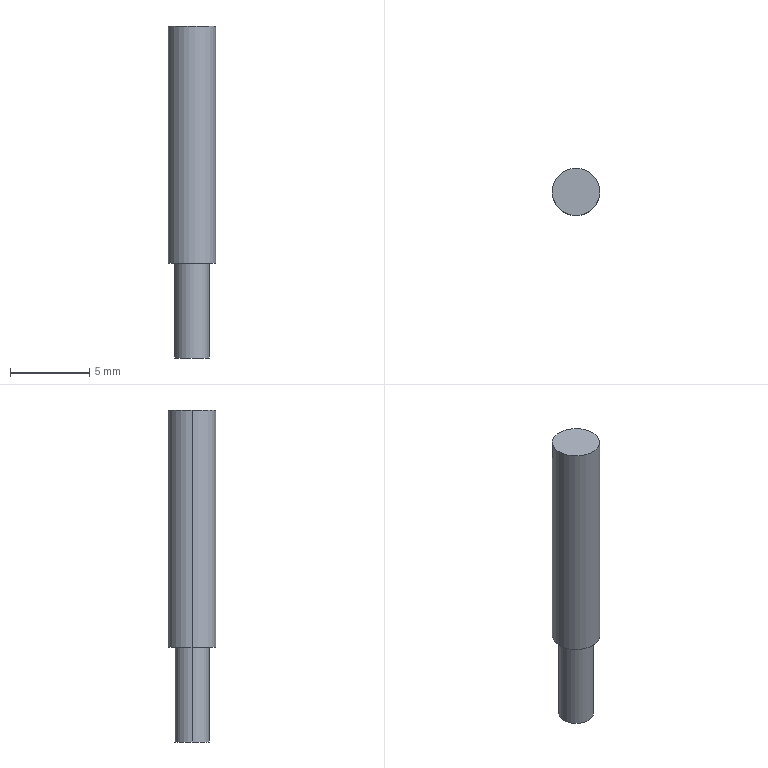Part | STEP file | through-beam fiber sensor FT-D321Q-M | 1 solid | 7 faces | box 3 x 3 x 21 mm | volume 128.837 mm3 | cylinder 4 | plane 3 | commonest cylinder face diameters 2.2 x2 3 x2
STEP:
#1=CARTESIAN_POINT('',(0.,0.,0.));
#2=DIRECTION('',(0.,0.,1.));
#3=DIRECTION('',(1.,0.,0.));
#4=AXIS2_PLACEMENT_3D('',#1,#2,#3);
#5=CARTESIAN_POINT('',(-1.1,0.,-6.));
#6=VERTEX_POINT('',#5);
#7=CARTESIAN_POINT('',(1.1,0.,-6.));
#8=VERTEX_POINT('',#7);
#9=CARTESIAN_POINT('',(0.,0.,-6.));
#10=DIRECTION('',(0.,0.,-1.));
#11=DIRECTION('',(-1.,0.,0.));
#12=AXIS2_PLACEMENT_3D('',#9,#10,#11);
#13=CIRCLE('',#12,1.1);
#14=CARTESIAN_POINT('',(0.,0.,-6.));
#15=DIRECTION('',(0.,0.,1.));
#16=DIRECTION('',(1.,0.,0.));
#17=AXIS2_PLACEMENT_3D('',#14,#15,#16);
#18=CYLINDRICAL_SURFACE('',#17,1.1);
#19=CARTESIAN_POINT('',(3.142,0.));
#20=DIRECTION('',(-1.,0.));
#21=VECTOR('',#20,1.);
#22=LINE('',#19,#21);
#23=(GEOMETRIC_REPRESENTATION_CONTEXT(2)PARAMETRIC_REPRESENTATION_CONTEXT()REPRESENTATION_CONTEXT('',''));
#24=DEFINITIONAL_REPRESENTATION('',(#22),#23);
#25=PCURVE('',#18,#24);
#26=CARTESIAN_POINT('',(0.,0.,-6.));
#27=DIRECTION('',(0.,0.,-1.));
#28=DIRECTION('',(-1.,0.,0.));
#29=AXIS2_PLACEMENT_3D('',#26,#27,#28);
#30=PLANE('',#29);
#31=CARTESIAN_POINT('',(0.,0.));
#32=DIRECTION('',(1.,0.));
#33=AXIS2_PLACEMENT_2D('',#31,#32);
#34=CIRCLE('',#33,1.1);
#35=(GEOMETRIC_REPRESENTATION_CONTEXT(2)PARAMETRIC_REPRESENTATION_CONTEXT()REPRESENTATION_CONTEXT('',''));
#36=DEFINITIONAL_REPRESENTATION('',(#34),#35);
#37=PCURVE('',#30,#36);
#38=SURFACE_CURVE('',#13,(#25,#37),.PCURVE_S1.);
#39=EDGE_CURVE('',#6,#8,#38,.T.);
#40=ORIENTED_EDGE('',*,*,#39,.F.);
#41=CARTESIAN_POINT('',(-1.1,0.,0.));
#42=VERTEX_POINT('',#41);
#43=CARTESIAN_POINT('',(-1.1,0.,-6.));
#44=DIRECTION('',(0.,0.,1.));
#45=VECTOR('',#44,1.);
#46=LINE('',#43,#45);
#47=CARTESIAN_POINT('',(3.142,0.));
#48=DIRECTION('',(0.,1.));
#49=VECTOR('',#48,1.);
#50=LINE('',#47,#49);
#51=(GEOMETRIC_REPRESENTATION_CONTEXT(2)PARAMETRIC_REPRESENTATION_CONTEXT()REPRESENTATION_CONTEXT('',''));
#52=DEFINITIONAL_REPRESENTATION('',(#50),#51);
#53=PCURVE('',#18,#52);
#54=CARTESIAN_POINT('',(0.,0.,-6.));
#55=DIRECTION('',(0.,0.,1.));
#56=DIRECTION('',(1.,0.,0.));
#57=AXIS2_PLACEMENT_3D('',#54,#55,#56);
#58=CYLINDRICAL_SURFACE('',#57,1.1);
#59=CARTESIAN_POINT('',(3.142,0.));
#60=DIRECTION('',(0.,1.));
#61=VECTOR('',#60,1.);
#62=LINE('',#59,#61);
#63=(GEOMETRIC_REPRESENTATION_CONTEXT(2)PARAMETRIC_REPRESENTATION_CONTEXT()REPRESENTATION_CONTEXT('',''));
#64=DEFINITIONAL_REPRESENTATION('',(#62),#63);
#65=PCURVE('',#58,#64);
#66=SURFACE_CURVE('',#46,(#53,#65),.PCURVE_S1.);
#67=EDGE_CURVE('',#6,#42,#66,.T.);
#68=ORIENTED_EDGE('',*,*,#67,.T.);
#69=CARTESIAN_POINT('',(1.1,0.,0.));
#70=VERTEX_POINT('',#69);
#71=CARTESIAN_POINT('',(0.,0.,0.));
#72=DIRECTION('',(0.,0.,-1.));
#73=DIRECTION('',(-1.,0.,0.));
#74=AXIS2_PLACEMENT_3D('',#71,#72,#73);
#75=CIRCLE('',#74,1.1);
#76=CARTESIAN_POINT('',(3.142,6.));
#77=DIRECTION('',(-1.,0.));
#78=VECTOR('',#77,1.);
#79=LINE('',#76,#78);
#80=(GEOMETRIC_REPRESENTATION_CONTEXT(2)PARAMETRIC_REPRESENTATION_CONTEXT()REPRESENTATION_CONTEXT('',''));
#81=DEFINITIONAL_REPRESENTATION('',(#79),#80);
#82=PCURVE('',#18,#81);
#83=CARTESIAN_POINT('',(0.,0.,0.));
#84=DIRECTION('',(0.,0.,1.));
#85=DIRECTION('',(1.,0.,0.));
#86=AXIS2_PLACEMENT_3D('',#83,#84,#85);
#87=PLANE('',#86);
#88=CARTESIAN_POINT('',(-1.1,0.));
#89=CARTESIAN_POINT('',(-1.1,1.905));
#90=CARTESIAN_POINT('',(0.55,0.9526));
#91=CARTESIAN_POINT('',(2.2,0.));
#92=CARTESIAN_POINT('',(0.55,-0.9526));
#93=CARTESIAN_POINT('',(-1.1,-1.905));
#94=CARTESIAN_POINT('',(-1.1,0.));
#95=(BOUNDED_CURVE()B_SPLINE_CURVE(2,(#88,#89,#90,#91,#92,#93,#94),.UNSPECIFIED.,.T.,.F.)B_SPLINE_CURVE_WITH_KNOTS((1,2,2,2,2,1),(-2.094,0.,2.094,4.189,6.283,8.378),.UNSPECIFIED.)CURVE()GEOMETRIC_REPRESENTATION_ITEM()RATIONAL_B_SPLINE_CURVE((1.,0.5,1.,0.5,1.,0.5,1.))REPRESENTATION_ITEM(''));
#96=(GEOMETRIC_REPRESENTATION_CONTEXT(2)PARAMETRIC_REPRESENTATION_CONTEXT()REPRESENTATION_CONTEXT('',''));
#97=DEFINITIONAL_REPRESENTATION('',(#95),#96);
#98=PCURVE('',#87,#97);
#99=SURFACE_CURVE('',#75,(#82,#98),.PCURVE_S1.);
#100=EDGE_CURVE('',#42,#70,#99,.T.);
#101=ORIENTED_EDGE('',*,*,#100,.T.);
#102=CARTESIAN_POINT('',(1.1,0.,-6.));
#103=DIRECTION('',(0.,0.,1.));
#104=VECTOR('',#103,1.);
#105=LINE('',#102,#104);
#106=CARTESIAN_POINT('',(0.,0.));
#107=DIRECTION('',(0.,1.));
#108=VECTOR('',#107,1.);
#109=LINE('',#106,#108);
#110=(GEOMETRIC_REPRESENTATION_CONTEXT(2)PARAMETRIC_REPRESENTATION_CONTEXT()REPRESENTATION_CONTEXT('',''));
#111=DEFINITIONAL_REPRESENTATION('',(#109),#110);
#112=PCURVE('',#18,#111);
#113=CARTESIAN_POINT('',(6.283,0.));
#114=DIRECTION('',(0.,1.));
#115=VECTOR('',#114,1.);
#116=LINE('',#113,#115);
#117=(GEOMETRIC_REPRESENTATION_CONTEXT(2)PARAMETRIC_REPRESENTATION_CONTEXT()REPRESENTATION_CONTEXT('',''));
#118=DEFINITIONAL_REPRESENTATION('',(#116),#117);
#119=PCURVE('',#58,#118);
#120=SURFACE_CURVE('',#105,(#112,#119),.PCURVE_S1.);
#121=EDGE_CURVE('',#8,#70,#120,.T.);
#122=ORIENTED_EDGE('',*,*,#121,.F.);
#123=EDGE_LOOP('',(#40,#68,#101,#122));
#124=FACE_BOUND('',#123,.T.);
#125=ADVANCED_FACE('',(#124),#18,.T.);
#126=CARTESIAN_POINT('',(1.5,0.,15.));
#127=VERTEX_POINT('',#126);
#128=CARTESIAN_POINT('',(-1.5,0.,15.));
#129=VERTEX_POINT('',#128);
#130=CARTESIAN_POINT('',(0.,0.,15.));
#131=DIRECTION('',(0.,0.,1.));
#132=DIRECTION('',(1.,0.,0.));
#133=AXIS2_PLACEMENT_3D('',#130,#131,#132);
#134=CIRCLE('',#133,1.5);
#135=CARTESIAN_POINT('',(0.,0.,15.));
#136=DIRECTION('',(0.,0.,-1.));
#137=DIRECTION('',(-1.,0.,0.));
#138=AXIS2_PLACEMENT_3D('',#135,#136,#137);
#139=CYLINDRICAL_SURFACE('',#138,1.5);
#140=CARTESIAN_POINT('',(3.142,0.));
#141=DIRECTION('',(-1.,0.));
#142=VECTOR('',#141,1.);
#143=LINE('',#140,#142);
#144=(GEOMETRIC_REPRESENTATION_CONTEXT(2)PARAMETRIC_REPRESENTATION_CONTEXT()REPRESENTATION_CONTEXT('',''));
#145=DEFINITIONAL_REPRESENTATION('',(#143),#144);
#146=PCURVE('',#139,#145);
#147=CARTESIAN_POINT('',(0.,0.,15.));
#148=DIRECTION('',(0.,0.,1.));
#149=DIRECTION('',(1.,0.,0.));
#150=AXIS2_PLACEMENT_3D('',#147,#148,#149);
#151=PLANE('',#150);
#152=CARTESIAN_POINT('',(0.,0.));
#153=DIRECTION('',(1.,0.));
#154=AXIS2_PLACEMENT_2D('',#152,#153);
#155=CIRCLE('',#154,1.5);
#156=(GEOMETRIC_REPRESENTATION_CONTEXT(2)PARAMETRIC_REPRESENTATION_CONTEXT()REPRESENTATION_CONTEXT('',''));
#157=DEFINITIONAL_REPRESENTATION('',(#155),#156);
#158=PCURVE('',#151,#157);
#159=SURFACE_CURVE('',#134,(#146,#158),.PCURVE_S1.);
#160=EDGE_CURVE('',#127,#129,#159,.T.);
#161=ORIENTED_EDGE('',*,*,#160,.F.);
#162=CARTESIAN_POINT('',(1.5,0.,0.));
#163=VERTEX_POINT('',#162);
#164=CARTESIAN_POINT('',(1.5,0.,15.));
#165=DIRECTION('',(0.,0.,-1.));
#166=VECTOR('',#165,1.);
#167=LINE('',#164,#166);
#168=CARTESIAN_POINT('',(3.142,0.));
#169=DIRECTION('',(0.,1.));
#170=VECTOR('',#169,1.);
#171=LINE('',#168,#170);
#172=(GEOMETRIC_REPRESENTATION_CONTEXT(2)PARAMETRIC_REPRESENTATION_CONTEXT()REPRESENTATION_CONTEXT('',''));
#173=DEFINITIONAL_REPRESENTATION('',(#171),#172);
#174=PCURVE('',#139,#173);
#175=CARTESIAN_POINT('',(0.,0.,15.));
#176=DIRECTION('',(0.,0.,-1.));
#177=DIRECTION('',(-1.,0.,0.));
#178=AXIS2_PLACEMENT_3D('',#175,#176,#177);
#179=CYLINDRICAL_SURFACE('',#178,1.5);
#180=CARTESIAN_POINT('',(3.142,0.));
#181=DIRECTION('',(0.,1.));
#182=VECTOR('',#181,1.);
#183=LINE('',#180,#182);
#184=(GEOMETRIC_REPRESENTATION_CONTEXT(2)PARAMETRIC_REPRESENTATION_CONTEXT()REPRESENTATION_CONTEXT('',''));
#185=DEFINITIONAL_REPRESENTATION('',(#183),#184);
#186=PCURVE('',#179,#185);
#187=SURFACE_CURVE('',#167,(#174,#186),.PCURVE_S1.);
#188=EDGE_CURVE('',#127,#163,#187,.T.);
#189=ORIENTED_EDGE('',*,*,#188,.T.);
#190=CARTESIAN_POINT('',(-1.5,0.,0.));
#191=VERTEX_POINT('',#190);
#192=CARTESIAN_POINT('',(0.,0.,0.));
#193=DIRECTION('',(0.,0.,1.));
#194=DIRECTION('',(1.,0.,0.));
#195=AXIS2_PLACEMENT_3D('',#192,#193,#194);
#196=CIRCLE('',#195,1.5);
#197=CARTESIAN_POINT('',(3.142,15.));
#198=DIRECTION('',(-1.,0.));
#199=VECTOR('',#198,1.);
#200=LINE('',#197,#199);
#201=(GEOMETRIC_REPRESENTATION_CONTEXT(2)PARAMETRIC_REPRESENTATION_CONTEXT()REPRESENTATION_CONTEXT('',''));
#202=DEFINITIONAL_REPRESENTATION('',(#200),#201);
#203=PCURVE('',#139,#202);
#204=CARTESIAN_POINT('',(0.,0.));
#205=DIRECTION('',(1.,0.));
#206=AXIS2_PLACEMENT_2D('',#204,#205);
#207=CIRCLE('',#206,1.5);
#208=(GEOMETRIC_REPRESENTATION_CONTEXT(2)PARAMETRIC_REPRESENTATION_CONTEXT()REPRESENTATION_CONTEXT('',''));
#209=DEFINITIONAL_REPRESENTATION('',(#207),#208);
#210=PCURVE('',#87,#209);
#211=SURFACE_CURVE('',#196,(#203,#210),.PCURVE_S1.);
#212=EDGE_CURVE('',#163,#191,#211,.T.);
#213=ORIENTED_EDGE('',*,*,#212,.T.);
#214=CARTESIAN_POINT('',(-1.5,0.,15.));
#215=DIRECTION('',(0.,0.,-1.));
#216=VECTOR('',#215,1.);
#217=LINE('',#214,#216);
#218=CARTESIAN_POINT('',(0.,0.));
#219=DIRECTION('',(0.,1.));
#220=VECTOR('',#219,1.);
#221=LINE('',#218,#220);
#222=(GEOMETRIC_REPRESENTATION_CONTEXT(2)PARAMETRIC_REPRESENTATION_CONTEXT()REPRESENTATION_CONTEXT('',''));
#223=DEFINITIONAL_REPRESENTATION('',(#221),#222);
#224=PCURVE('',#139,#223);
#225=CARTESIAN_POINT('',(6.283,0.));
#226=DIRECTION('',(0.,1.));
#227=VECTOR('',#226,1.);
#228=LINE('',#225,#227);
#229=(GEOMETRIC_REPRESENTATION_CONTEXT(2)PARAMETRIC_REPRESENTATION_CONTEXT()REPRESENTATION_CONTEXT('',''));
#230=DEFINITIONAL_REPRESENTATION('',(#228),#229);
#231=PCURVE('',#179,#230);
#232=SURFACE_CURVE('',#217,(#224,#231),.PCURVE_S1.);
#233=EDGE_CURVE('',#129,#191,#232,.T.);
#234=ORIENTED_EDGE('',*,*,#233,.F.);
#235=EDGE_LOOP('',(#161,#189,#213,#234));
#236=FACE_BOUND('',#235,.T.);
#237=ADVANCED_FACE('',(#236),#139,.T.);
#238=ORIENTED_EDGE('',*,*,#188,.F.);
#239=CARTESIAN_POINT('',(0.,0.,15.));
#240=DIRECTION('',(0.,0.,1.));
#241=DIRECTION('',(1.,0.,0.));
#242=AXIS2_PLACEMENT_3D('',#239,#240,#241);
#243=CIRCLE('',#242,1.5);
#244=CARTESIAN_POINT('',(9.425,0.));
#245=DIRECTION('',(-1.,0.));
#246=VECTOR('',#245,1.);
#247=LINE('',#244,#246);
#248=(GEOMETRIC_REPRESENTATION_CONTEXT(2)PARAMETRIC_REPRESENTATION_CONTEXT()REPRESENTATION_CONTEXT('',''));
#249=DEFINITIONAL_REPRESENTATION('',(#247),#248);
#250=PCURVE('',#179,#249);
#251=CARTESIAN_POINT('',(0.,0.));
#252=DIRECTION('',(1.,0.));
#253=AXIS2_PLACEMENT_2D('',#251,#252);
#254=CIRCLE('',#253,1.5);
#255=(GEOMETRIC_REPRESENTATION_CONTEXT(2)PARAMETRIC_REPRESENTATION_CONTEXT()REPRESENTATION_CONTEXT('',''));
#256=DEFINITIONAL_REPRESENTATION('',(#254),#255);
#257=PCURVE('',#151,#256);
#258=SURFACE_CURVE('',#243,(#250,#257),.PCURVE_S1.);
#259=EDGE_CURVE('',#129,#127,#258,.T.);
#260=ORIENTED_EDGE('',*,*,#259,.F.);
#261=ORIENTED_EDGE('',*,*,#233,.T.);
#262=CARTESIAN_POINT('',(0.,0.,0.));
#263=DIRECTION('',(0.,0.,1.));
#264=DIRECTION('',(1.,0.,0.));
#265=AXIS2_PLACEMENT_3D('',#262,#263,#264);
#266=CIRCLE('',#265,1.5);
#267=CARTESIAN_POINT('',(9.425,15.));
#268=DIRECTION('',(-1.,0.));
#269=VECTOR('',#268,1.);
#270=LINE('',#267,#269);
#271=(GEOMETRIC_REPRESENTATION_CONTEXT(2)PARAMETRIC_REPRESENTATION_CONTEXT()REPRESENTATION_CONTEXT('',''));
#272=DEFINITIONAL_REPRESENTATION('',(#270),#271);
#273=PCURVE('',#179,#272);
#274=CARTESIAN_POINT('',(0.,0.));
#275=DIRECTION('',(1.,0.));
#276=AXIS2_PLACEMENT_2D('',#274,#275);
#277=CIRCLE('',#276,1.5);
#278=(GEOMETRIC_REPRESENTATION_CONTEXT(2)PARAMETRIC_REPRESENTATION_CONTEXT()REPRESENTATION_CONTEXT('',''));
#279=DEFINITIONAL_REPRESENTATION('',(#277),#278);
#280=PCURVE('',#87,#279);
#281=SURFACE_CURVE('',#266,(#273,#280),.PCURVE_S1.);
#282=EDGE_CURVE('',#191,#163,#281,.T.);
#283=ORIENTED_EDGE('',*,*,#282,.T.);
#284=EDGE_LOOP('',(#238,#260,#261,#283));
#285=FACE_BOUND('',#284,.T.);
#286=ADVANCED_FACE('',(#285),#179,.T.);
#287=ORIENTED_EDGE('',*,*,#259,.T.);
#288=ORIENTED_EDGE('',*,*,#160,.T.);
#289=EDGE_LOOP('',(#287,#288));
#290=FACE_BOUND('',#289,.T.);
#291=ADVANCED_FACE('',(#290),#151,.T.);
#292=CARTESIAN_POINT('',(0.,0.,0.));
#293=DIRECTION('',(0.,0.,-1.));
#294=DIRECTION('',(-1.,0.,0.));
#295=AXIS2_PLACEMENT_3D('',#292,#293,#294);
#296=CIRCLE('',#295,1.1);
#297=CARTESIAN_POINT('',(-1.1,0.));
#298=CARTESIAN_POINT('',(-1.1,1.905));
#299=CARTESIAN_POINT('',(0.55,0.9526));
#300=CARTESIAN_POINT('',(2.2,0.));
#301=CARTESIAN_POINT('',(0.55,-0.9526));
#302=CARTESIAN_POINT('',(-1.1,-1.905));
#303=CARTESIAN_POINT('',(-1.1,0.));
#304=(BOUNDED_CURVE()B_SPLINE_CURVE(2,(#297,#298,#299,#300,#301,#302,#303),.UNSPECIFIED.,.T.,.F.)B_SPLINE_CURVE_WITH_KNOTS((1,2,2,2,2,1),(-2.094,0.,2.094,4.189,6.283,8.378),.UNSPECIFIED.)CURVE()GEOMETRIC_REPRESENTATION_ITEM()RATIONAL_B_SPLINE_CURVE((1.,0.5,1.,0.5,1.,0.5,1.))REPRESENTATION_ITEM(''));
#305=(GEOMETRIC_REPRESENTATION_CONTEXT(2)PARAMETRIC_REPRESENTATION_CONTEXT()REPRESENTATION_CONTEXT('',''));
#306=DEFINITIONAL_REPRESENTATION('',(#304),#305);
#307=PCURVE('',#87,#306);
#308=CARTESIAN_POINT('',(9.425,6.));
#309=DIRECTION('',(-1.,0.));
#310=VECTOR('',#309,1.);
#311=LINE('',#308,#310);
#312=(GEOMETRIC_REPRESENTATION_CONTEXT(2)PARAMETRIC_REPRESENTATION_CONTEXT()REPRESENTATION_CONTEXT('',''));
#313=DEFINITIONAL_REPRESENTATION('',(#311),#312);
#314=PCURVE('',#58,#313);
#315=SURFACE_CURVE('',#296,(#307,#314),.PCURVE_S1.);
#316=EDGE_CURVE('',#70,#42,#315,.T.);
#317=ORIENTED_EDGE('',*,*,#316,.F.);
#318=ORIENTED_EDGE('',*,*,#100,.F.);
#319=EDGE_LOOP('',(#317,#318));
#320=FACE_BOUND('',#319,.T.);
#321=ORIENTED_EDGE('',*,*,#282,.F.);
#322=ORIENTED_EDGE('',*,*,#212,.F.);
#323=EDGE_LOOP('',(#321,#322));
#324=FACE_BOUND('',#323,.T.);
#325=ADVANCED_FACE('',(#320,#324),#87,.F.);
#326=ORIENTED_EDGE('',*,*,#67,.F.);
#327=CARTESIAN_POINT('',(0.,0.,-6.));
#328=DIRECTION('',(0.,0.,-1.));
#329=DIRECTION('',(-1.,0.,0.));
#330=AXIS2_PLACEMENT_3D('',#327,#328,#329);
#331=CIRCLE('',#330,1.1);
#332=CARTESIAN_POINT('',(9.425,0.));
#333=DIRECTION('',(-1.,0.));
#334=VECTOR('',#333,1.);
#335=LINE('',#332,#334);
#336=(GEOMETRIC_REPRESENTATION_CONTEXT(2)PARAMETRIC_REPRESENTATION_CONTEXT()REPRESENTATION_CONTEXT('',''));
#337=DEFINITIONAL_REPRESENTATION('',(#335),#336);
#338=PCURVE('',#58,#337);
#339=CARTESIAN_POINT('',(0.,0.));
#340=DIRECTION('',(1.,0.));
#341=AXIS2_PLACEMENT_2D('',#339,#340);
#342=CIRCLE('',#341,1.1);
#343=(GEOMETRIC_REPRESENTATION_CONTEXT(2)PARAMETRIC_REPRESENTATION_CONTEXT()REPRESENTATION_CONTEXT('',''));
#344=DEFINITIONAL_REPRESENTATION('',(#342),#343);
#345=PCURVE('',#30,#344);
#346=SURFACE_CURVE('',#331,(#338,#345),.PCURVE_S1.);
#347=EDGE_CURVE('',#8,#6,#346,.T.);
#348=ORIENTED_EDGE('',*,*,#347,.F.);
#349=ORIENTED_EDGE('',*,*,#121,.T.);
#350=ORIENTED_EDGE('',*,*,#316,.T.);
#351=EDGE_LOOP('',(#326,#348,#349,#350));
#352=FACE_BOUND('',#351,.T.);
#353=ADVANCED_FACE('',(#352),#58,.T.);
#354=ORIENTED_EDGE('',*,*,#347,.T.);
#355=ORIENTED_EDGE('',*,*,#39,.T.);
#356=EDGE_LOOP('',(#354,#355));
#357=FACE_BOUND('',#356,.T.);
#358=ADVANCED_FACE('',(#357),#30,.T.);
#359=CLOSED_SHELL('',(#125,#237,#286,#291,#325,#353,#358));
#360=MANIFOLD_SOLID_BREP('',#359);
#361=(LENGTH_UNIT()NAMED_UNIT(*)SI_UNIT(.MILLI.,.METRE.));
#362=UNCERTAINTY_MEASURE_WITH_UNIT(LENGTH_MEASURE(0.0000001),#361,'','');
#363=(NAMED_UNIT(*)PLANE_ANGLE_UNIT()SI_UNIT($,.RADIAN.));
#364=(NAMED_UNIT(*)SI_UNIT($,.STERADIAN.)SOLID_ANGLE_UNIT());
#365=(GEOMETRIC_REPRESENTATION_CONTEXT(3)GLOBAL_UNCERTAINTY_ASSIGNED_CONTEXT((#362))GLOBAL_UNIT_ASSIGNED_CONTEXT((#361,#363,#364))REPRESENTATION_CONTEXT('',''));
#366=ADVANCED_BREP_SHAPE_REPRESENTATION('',(#4,#360),#365);